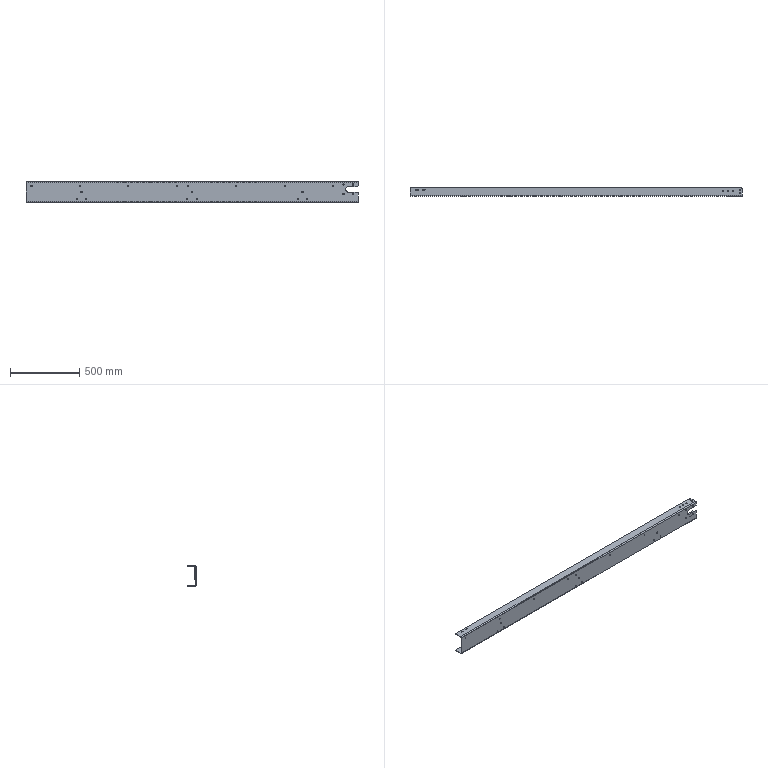Part | STEP file | UPPER.FRAME.2.stp | 1 solid | 114 faces | box 2400 x 60 x 150 mm | volume 2791918 mm3 | spline 65 | cylinder 36 | plane 13 | commonest cylinder face diameters 7 x10 8 x8 9 x8 11 x6 6 x2 15 x2